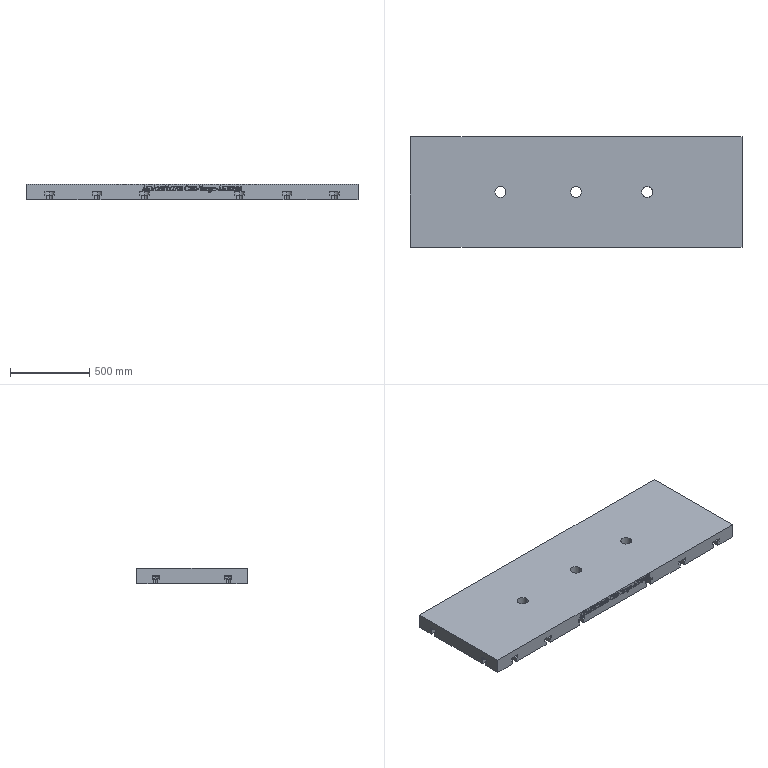Part | CATIA | 1 solid | 784 faces | box 2100 x 700 x 95 mm | volume 132752319 mm3 | other 347 | plane 322 | cylinder 87 | torus 16 | spline 8 | cone 4 | commonest cylinder face diameters 36 x23 60 x23 2 x8 5 x8 28 x8 46 x8